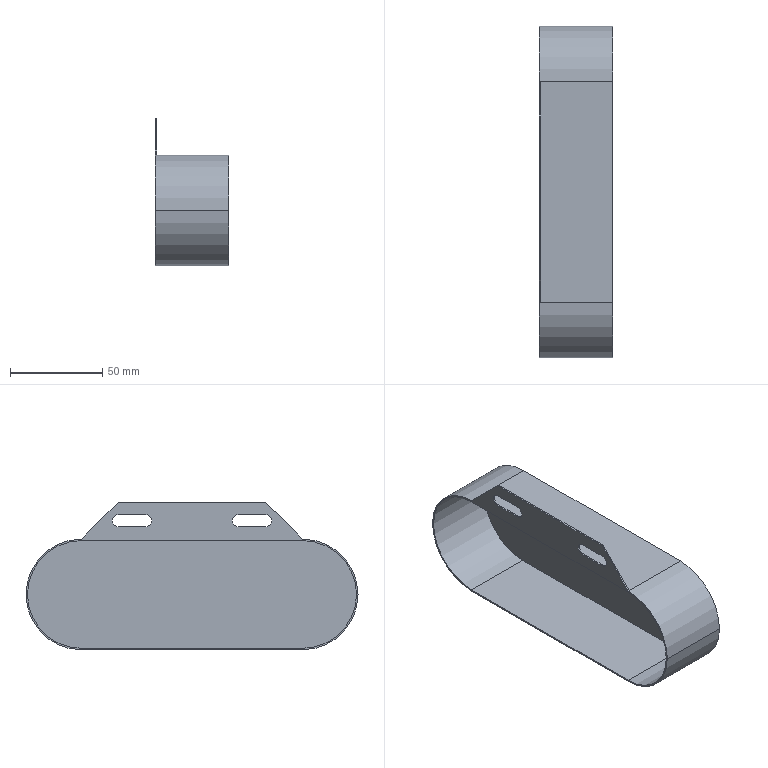Part | STEP file | 02-23 Sprocket cover | 1 solid | 25 faces | box 40 x 180 x 80 mm | volume 22772 mm3 | plane 15 | cylinder 10 | commonest cylinder face diameters 6.5 x4 58.4 x3 60 x3